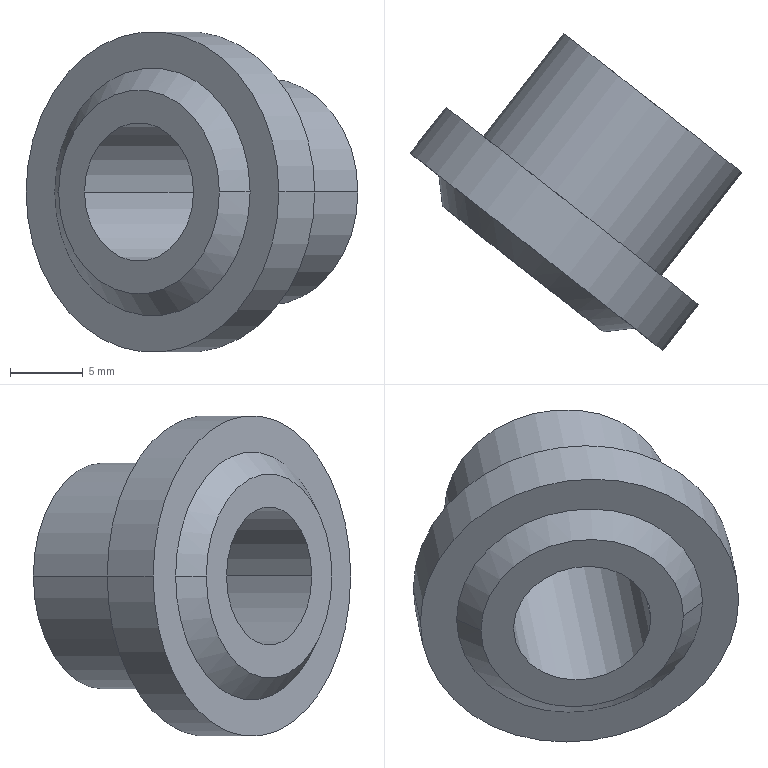Part | STEP file | VALVE_2PARTV11 | 1 solid | 12 faces | box 22.76 x 21.764 x 22 mm | volume 2471 mm3 | cylinder 6 | plane 4 | cone 2 | commonest cylinder face diameters 9.5 x2 15.5 x2 22 x2
STEP:
#1=CARTESIAN_POINT('',(0.,0.,0.));
#2=DIRECTION('',(0.,0.,1.));
#3=DIRECTION('',(1.,0.,0.));
#4=AXIS2_PLACEMENT_3D('',#1,#2,#3);
#5=CARTESIAN_POINT('',(-4.617,4.509,0.));
#6=VERTEX_POINT('',#5);
#7=CARTESIAN_POINT('',(12.719,-9.035,0.));
#8=VERTEX_POINT('',#7);
#9=CARTESIAN_POINT('',(4.051,-2.263,0.));
#10=DIRECTION('',(0.6157,0.788,0.));
#11=DIRECTION('',(-0.788,0.6157,0.));
#12=AXIS2_PLACEMENT_3D('',#9,#10,#11);
#13=CIRCLE('',#12,11.);
#14=CARTESIAN_POINT('',(2.204,-4.627,0.));
#15=DIRECTION('',(0.6157,0.788,0.));
#16=DIRECTION('',(-0.788,0.6157,0.));
#17=AXIS2_PLACEMENT_3D('',#14,#15,#16);
#18=CYLINDRICAL_SURFACE('',#17,11.);
#19=CARTESIAN_POINT('',(0.,3.));
#20=DIRECTION('',(1.,0.));
#21=VECTOR('',#20,1.);
#22=LINE('',#19,#21);
#23=(GEOMETRIC_REPRESENTATION_CONTEXT(2)PARAMETRIC_REPRESENTATION_CONTEXT()REPRESENTATION_CONTEXT('',''));
#24=DEFINITIONAL_REPRESENTATION('',(#22),#23);
#25=PCURVE('',#18,#24);
#26=CARTESIAN_POINT('',(-4.617,4.509,0.));
#27=DIRECTION('',(-0.6157,-0.788,0.));
#28=DIRECTION('',(0.788,-0.6157,0.));
#29=AXIS2_PLACEMENT_3D('',#26,#27,#28);
#30=PLANE('',#29);
#31=CARTESIAN_POINT('',(0.,0.));
#32=CARTESIAN_POINT('',(0.,19.053));
#33=CARTESIAN_POINT('',(16.5,9.526));
#34=CARTESIAN_POINT('',(33.,0.));
#35=CARTESIAN_POINT('',(16.5,-9.526));
#36=CARTESIAN_POINT('',(0.,-19.053));
#37=CARTESIAN_POINT('',(0.,0.));
#38=(BOUNDED_CURVE()B_SPLINE_CURVE(2,(#31,#32,#33,#34,#35,#36,#37),.UNSPECIFIED.,.T.,.F.)B_SPLINE_CURVE_WITH_KNOTS((1,2,2,2,2,1),(-2.094,0.,2.094,4.189,6.283,8.378),.UNSPECIFIED.)CURVE()GEOMETRIC_REPRESENTATION_ITEM()RATIONAL_B_SPLINE_CURVE((1.,0.5,1.,0.5,1.,0.5,1.))REPRESENTATION_ITEM(''));
#39=(GEOMETRIC_REPRESENTATION_CONTEXT(2)PARAMETRIC_REPRESENTATION_CONTEXT()REPRESENTATION_CONTEXT('',''));
#40=DEFINITIONAL_REPRESENTATION('',(#38),#39);
#41=PCURVE('',#30,#40);
#42=SURFACE_CURVE('',#13,(#25,#41),.PCURVE_S1.);
#43=EDGE_CURVE('',#6,#8,#42,.T.);
#44=ORIENTED_EDGE('',*,*,#43,.T.);
#45=CARTESIAN_POINT('',(15.182,-5.883,0.));
#46=VERTEX_POINT('',#45);
#47=CARTESIAN_POINT('',(10.872,-11.399,0.));
#48=DIRECTION('',(0.6157,0.788,0.));
#49=VECTOR('',#48,1.);
#50=LINE('',#47,#49);
#51=CARTESIAN_POINT('',(3.142,0.));
#52=DIRECTION('',(0.,1.));
#53=VECTOR('',#52,1.);
#54=LINE('',#51,#53);
#55=(GEOMETRIC_REPRESENTATION_CONTEXT(2)PARAMETRIC_REPRESENTATION_CONTEXT()REPRESENTATION_CONTEXT('',''));
#56=DEFINITIONAL_REPRESENTATION('',(#54),#55);
#57=PCURVE('',#18,#56);
#58=CARTESIAN_POINT('',(2.204,-4.627,0.));
#59=DIRECTION('',(0.6157,0.788,0.));
#60=DIRECTION('',(-0.788,0.6157,0.));
#61=AXIS2_PLACEMENT_3D('',#58,#59,#60);
#62=CYLINDRICAL_SURFACE('',#61,11.);
#63=CARTESIAN_POINT('',(3.142,0.));
#64=DIRECTION('',(0.,1.));
#65=VECTOR('',#64,1.);
#66=LINE('',#63,#65);
#67=(GEOMETRIC_REPRESENTATION_CONTEXT(2)PARAMETRIC_REPRESENTATION_CONTEXT()REPRESENTATION_CONTEXT('',''));
#68=DEFINITIONAL_REPRESENTATION('',(#66),#67);
#69=PCURVE('',#62,#68);
#70=SURFACE_CURVE('',#50,(#57,#69),.PCURVE_S1.);
#71=EDGE_CURVE('',#8,#46,#70,.T.);
#72=ORIENTED_EDGE('',*,*,#71,.T.);
#73=CARTESIAN_POINT('',(-2.155,7.661,0.));
#74=VERTEX_POINT('',#73);
#75=CARTESIAN_POINT('',(6.513,0.889,0.));
#76=DIRECTION('',(0.6157,0.788,0.));
#77=DIRECTION('',(-0.788,0.6157,0.));
#78=AXIS2_PLACEMENT_3D('',#75,#76,#77);
#79=CIRCLE('',#78,11.);
#80=CARTESIAN_POINT('',(0.,7.));
#81=DIRECTION('',(1.,0.));
#82=VECTOR('',#81,1.);
#83=LINE('',#80,#82);
#84=(GEOMETRIC_REPRESENTATION_CONTEXT(2)PARAMETRIC_REPRESENTATION_CONTEXT()REPRESENTATION_CONTEXT('',''));
#85=DEFINITIONAL_REPRESENTATION('',(#83),#84);
#86=PCURVE('',#18,#85);
#87=CARTESIAN_POINT('',(0.4063,5.66,0.));
#88=DIRECTION('',(0.6157,0.788,0.));
#89=DIRECTION('',(-0.788,0.6157,0.));
#90=AXIS2_PLACEMENT_3D('',#87,#88,#89);
#91=PLANE('',#90);
#92=CARTESIAN_POINT('',(-7.75,0.));
#93=DIRECTION('',(1.,0.));
#94=AXIS2_PLACEMENT_2D('',#92,#93);
#95=CIRCLE('',#94,11.);
#96=(GEOMETRIC_REPRESENTATION_CONTEXT(2)PARAMETRIC_REPRESENTATION_CONTEXT()REPRESENTATION_CONTEXT('',''));
#97=DEFINITIONAL_REPRESENTATION('',(#95),#96);
#98=PCURVE('',#91,#97);
#99=SURFACE_CURVE('',#79,(#86,#98),.PCURVE_S1.);
#100=EDGE_CURVE('',#74,#46,#99,.T.);
#101=ORIENTED_EDGE('',*,*,#100,.F.);
#102=CARTESIAN_POINT('',(-6.464,2.145,0.));
#103=DIRECTION('',(0.6157,0.788,0.));
#104=VECTOR('',#103,1.);
#105=LINE('',#102,#104);
#106=CARTESIAN_POINT('',(0.,0.));
#107=DIRECTION('',(0.,1.));
#108=VECTOR('',#107,1.);
#109=LINE('',#106,#108);
#110=(GEOMETRIC_REPRESENTATION_CONTEXT(2)PARAMETRIC_REPRESENTATION_CONTEXT()REPRESENTATION_CONTEXT('',''));
#111=DEFINITIONAL_REPRESENTATION('',(#109),#110);
#112=PCURVE('',#18,#111);
#113=CARTESIAN_POINT('',(6.283,0.));
#114=DIRECTION('',(0.,1.));
#115=VECTOR('',#114,1.);
#116=LINE('',#113,#115);
#117=(GEOMETRIC_REPRESENTATION_CONTEXT(2)PARAMETRIC_REPRESENTATION_CONTEXT()REPRESENTATION_CONTEXT('',''));
#118=DEFINITIONAL_REPRESENTATION('',(#116),#117);
#119=PCURVE('',#62,#118);
#120=SURFACE_CURVE('',#105,(#112,#119),.PCURVE_S1.);
#121=EDGE_CURVE('',#6,#74,#120,.T.);
#122=ORIENTED_EDGE('',*,*,#121,.F.);
#123=EDGE_LOOP('',(#44,#72,#101,#122));
#124=FACE_BOUND('',#123,.T.);
#125=ADVANCED_FACE('',(#124),#18,.T.);
#126=CARTESIAN_POINT('',(0.4063,5.66,0.));
#127=VERTEX_POINT('',#126);
#128=CARTESIAN_POINT('',(12.62,-3.882,0.));
#129=VERTEX_POINT('',#128);
#130=CARTESIAN_POINT('',(6.513,0.889,0.));
#131=DIRECTION('',(0.6157,0.788,0.));
#132=DIRECTION('',(-0.788,0.6157,0.));
#133=AXIS2_PLACEMENT_3D('',#130,#131,#132);
#134=CIRCLE('',#133,7.75);
#135=CARTESIAN_POINT('',(2.204,-4.627,0.));
#136=DIRECTION('',(0.6157,0.788,0.));
#137=DIRECTION('',(-0.788,0.6157,0.));
#138=AXIS2_PLACEMENT_3D('',#135,#136,#137);
#139=CYLINDRICAL_SURFACE('',#138,7.75);
#140=CARTESIAN_POINT('',(0.,7.));
#141=DIRECTION('',(1.,0.));
#142=VECTOR('',#141,1.);
#143=LINE('',#140,#142);
#144=(GEOMETRIC_REPRESENTATION_CONTEXT(2)PARAMETRIC_REPRESENTATION_CONTEXT()REPRESENTATION_CONTEXT('',''));
#145=DEFINITIONAL_REPRESENTATION('',(#143),#144);
#146=PCURVE('',#139,#145);
#147=CARTESIAN_POINT('',(-7.75,0.));
#148=DIRECTION('',(1.,0.));
#149=AXIS2_PLACEMENT_2D('',#147,#148);
#150=CIRCLE('',#149,7.75);
#151=(GEOMETRIC_REPRESENTATION_CONTEXT(2)PARAMETRIC_REPRESENTATION_CONTEXT()REPRESENTATION_CONTEXT('',''));
#152=DEFINITIONAL_REPRESENTATION('',(#150),#151);
#153=PCURVE('',#91,#152);
#154=SURFACE_CURVE('',#134,(#146,#153),.PCURVE_S1.);
#155=EDGE_CURVE('',#127,#129,#154,.T.);
#156=ORIENTED_EDGE('',*,*,#155,.T.);
#157=CARTESIAN_POINT('',(18.143,3.186,0.));
#158=VERTEX_POINT('',#157);
#159=CARTESIAN_POINT('',(8.311,-9.398,0.));
#160=DIRECTION('',(0.6157,0.788,0.));
#161=VECTOR('',#160,1.);
#162=LINE('',#159,#161);
#163=CARTESIAN_POINT('',(3.142,0.));
#164=DIRECTION('',(0.,1.));
#165=VECTOR('',#164,1.);
#166=LINE('',#163,#165);
#167=(GEOMETRIC_REPRESENTATION_CONTEXT(2)PARAMETRIC_REPRESENTATION_CONTEXT()REPRESENTATION_CONTEXT('',''));
#168=DEFINITIONAL_REPRESENTATION('',(#166),#167);
#169=PCURVE('',#139,#168);
#170=CARTESIAN_POINT('',(2.204,-4.627,0.));
#171=DIRECTION('',(0.6157,0.788,0.));
#172=DIRECTION('',(-0.788,0.6157,0.));
#173=AXIS2_PLACEMENT_3D('',#170,#171,#172);
#174=CYLINDRICAL_SURFACE('',#173,7.75);
#175=CARTESIAN_POINT('',(3.142,0.));
#176=DIRECTION('',(0.,1.));
#177=VECTOR('',#176,1.);
#178=LINE('',#175,#177);
#179=(GEOMETRIC_REPRESENTATION_CONTEXT(2)PARAMETRIC_REPRESENTATION_CONTEXT()REPRESENTATION_CONTEXT('',''));
#180=DEFINITIONAL_REPRESENTATION('',(#178),#179);
#181=PCURVE('',#174,#180);
#182=SURFACE_CURVE('',#162,(#169,#181),.PCURVE_S1.);
#183=EDGE_CURVE('',#129,#158,#182,.T.);
#184=ORIENTED_EDGE('',*,*,#183,.T.);
#185=CARTESIAN_POINT('',(5.929,12.728,0.));
#186=VERTEX_POINT('',#185);
#187=CARTESIAN_POINT('',(12.036,7.957,0.));
#188=DIRECTION('',(0.6157,0.788,0.));
#189=DIRECTION('',(-0.788,0.6157,0.));
#190=AXIS2_PLACEMENT_3D('',#187,#188,#189);
#191=CIRCLE('',#190,7.75);
#192=CARTESIAN_POINT('',(0.,15.97));
#193=DIRECTION('',(1.,0.));
#194=VECTOR('',#193,1.);
#195=LINE('',#192,#194);
#196=(GEOMETRIC_REPRESENTATION_CONTEXT(2)PARAMETRIC_REPRESENTATION_CONTEXT()REPRESENTATION_CONTEXT('',''));
#197=DEFINITIONAL_REPRESENTATION('',(#195),#196);
#198=PCURVE('',#139,#197);
#199=CARTESIAN_POINT('',(8.293,10.882,0.));
#200=DIRECTION('',(0.6157,0.788,0.));
#201=DIRECTION('',(-0.788,0.6157,0.));
#202=AXIS2_PLACEMENT_3D('',#199,#200,#201);
#203=PLANE('',#202);
#204=CARTESIAN_POINT('',(-4.75,0.));
#205=DIRECTION('',(1.,0.));
#206=AXIS2_PLACEMENT_2D('',#204,#205);
#207=CIRCLE('',#206,7.75);
#208=(GEOMETRIC_REPRESENTATION_CONTEXT(2)PARAMETRIC_REPRESENTATION_CONTEXT()REPRESENTATION_CONTEXT('',''));
#209=DEFINITIONAL_REPRESENTATION('',(#207),#208);
#210=PCURVE('',#203,#209);
#211=SURFACE_CURVE('',#191,(#198,#210),.PCURVE_S1.);
#212=EDGE_CURVE('',#186,#158,#211,.T.);
#213=ORIENTED_EDGE('',*,*,#212,.F.);
#214=CARTESIAN_POINT('',(-3.903,0.1443,0.));
#215=DIRECTION('',(0.6157,0.788,0.));
#216=VECTOR('',#215,1.);
#217=LINE('',#214,#216);
#218=CARTESIAN_POINT('',(0.,0.));
#219=DIRECTION('',(0.,1.));
#220=VECTOR('',#219,1.);
#221=LINE('',#218,#220);
#222=(GEOMETRIC_REPRESENTATION_CONTEXT(2)PARAMETRIC_REPRESENTATION_CONTEXT()REPRESENTATION_CONTEXT('',''));
#223=DEFINITIONAL_REPRESENTATION('',(#221),#222);
#224=PCURVE('',#139,#223);
#225=CARTESIAN_POINT('',(6.283,0.));
#226=DIRECTION('',(0.,1.));
#227=VECTOR('',#226,1.);
#228=LINE('',#225,#227);
#229=(GEOMETRIC_REPRESENTATION_CONTEXT(2)PARAMETRIC_REPRESENTATION_CONTEXT()REPRESENTATION_CONTEXT('',''));
#230=DEFINITIONAL_REPRESENTATION('',(#228),#229);
#231=PCURVE('',#174,#230);
#232=SURFACE_CURVE('',#217,(#224,#231),.PCURVE_S1.);
#233=EDGE_CURVE('',#127,#186,#232,.T.);
#234=ORIENTED_EDGE('',*,*,#233,.F.);
#235=EDGE_LOOP('',(#156,#184,#213,#234));
#236=FACE_BOUND('',#235,.T.);
#237=ADVANCED_FACE('',(#236),#139,.T.);
#238=CARTESIAN_POINT('',(-0.6158,-0.5207,0.));
#239=VERTEX_POINT('',#238);
#240=CARTESIAN_POINT('',(8.293,10.882,0.));
#241=VERTEX_POINT('',#240);
#242=CARTESIAN_POINT('',(-1.539,-1.703,0.));
#243=DIRECTION('',(0.6157,0.788,0.));
#244=VECTOR('',#243,1.);
#245=LINE('',#242,#244);
#246=CARTESIAN_POINT('',(2.204,-4.627,0.));
#247=DIRECTION('',(0.6157,0.788,0.));
#248=DIRECTION('',(-0.788,0.6157,0.));
#249=AXIS2_PLACEMENT_3D('',#246,#247,#248);
#250=CYLINDRICAL_SURFACE('',#249,4.75);
#251=CARTESIAN_POINT('',(6.283,0.));
#252=DIRECTION('',(0.,1.));
#253=VECTOR('',#252,1.);
#254=LINE('',#251,#253);
#255=(GEOMETRIC_REPRESENTATION_CONTEXT(2)PARAMETRIC_REPRESENTATION_CONTEXT()REPRESENTATION_CONTEXT('',''));
#256=DEFINITIONAL_REPRESENTATION('',(#254),#255);
#257=PCURVE('',#250,#256);
#258=CARTESIAN_POINT('',(2.204,-4.627,0.));
#259=DIRECTION('',(0.6157,0.788,0.));
#260=DIRECTION('',(-0.788,0.6157,0.));
#261=AXIS2_PLACEMENT_3D('',#258,#259,#260);
#262=CYLINDRICAL_SURFACE('',#261,4.75);
#263=CARTESIAN_POINT('',(0.,0.));
#264=DIRECTION('',(0.,1.));
#265=VECTOR('',#264,1.);
#266=LINE('',#263,#265);
#267=(GEOMETRIC_REPRESENTATION_CONTEXT(2)PARAMETRIC_REPRESENTATION_CONTEXT()REPRESENTATION_CONTEXT('',''));
#268=DEFINITIONAL_REPRESENTATION('',(#266),#267);
#269=PCURVE('',#262,#268);
#270=SURFACE_CURVE('',#245,(#257,#269),.PCURVE_S1.);
#271=EDGE_CURVE('',#239,#241,#270,.T.);
#272=ORIENTED_EDGE('',*,*,#271,.T.);
#273=CARTESIAN_POINT('',(15.779,5.033,0.));
#274=VERTEX_POINT('',#273);
#275=CARTESIAN_POINT('',(12.036,7.957,0.));
#276=DIRECTION('',(0.6157,0.788,0.));
#277=DIRECTION('',(-0.788,0.6157,0.));
#278=AXIS2_PLACEMENT_3D('',#275,#276,#277);
#279=CIRCLE('',#278,4.75);
#280=CARTESIAN_POINT('',(0.,15.97));
#281=DIRECTION('',(1.,0.));
#282=VECTOR('',#281,1.);
#283=LINE('',#280,#282);
#284=(GEOMETRIC_REPRESENTATION_CONTEXT(2)PARAMETRIC_REPRESENTATION_CONTEXT()REPRESENTATION_CONTEXT('',''));
#285=DEFINITIONAL_REPRESENTATION('',(#283),#284);
#286=PCURVE('',#250,#285);
#287=CARTESIAN_POINT('',(-4.75,0.));
#288=DIRECTION('',(1.,0.));
#289=AXIS2_PLACEMENT_2D('',#287,#288);
#290=CIRCLE('',#289,4.75);
#291=(GEOMETRIC_REPRESENTATION_CONTEXT(2)PARAMETRIC_REPRESENTATION_CONTEXT()REPRESENTATION_CONTEXT('',''));
#292=DEFINITIONAL_REPRESENTATION('',(#290),#291);
#293=PCURVE('',#203,#292);
#294=SURFACE_CURVE('',#279,(#286,#293),.PCURVE_S1.);
#295=EDGE_CURVE('',#274,#241,#294,.T.);
#296=ORIENTED_EDGE('',*,*,#295,.F.);
#297=CARTESIAN_POINT('',(6.87,-6.369,0.));
#298=VERTEX_POINT('',#297);
#299=CARTESIAN_POINT('',(5.947,-7.551,0.));
#300=DIRECTION('',(0.6157,0.788,0.));
#301=VECTOR('',#300,1.);
#302=LINE('',#299,#301);
#303=CARTESIAN_POINT('',(3.142,0.));
#304=DIRECTION('',(0.,1.));
#305=VECTOR('',#304,1.);
#306=LINE('',#303,#305);
#307=(GEOMETRIC_REPRESENTATION_CONTEXT(2)PARAMETRIC_REPRESENTATION_CONTEXT()REPRESENTATION_CONTEXT('',''));
#308=DEFINITIONAL_REPRESENTATION('',(#306),#307);
#309=PCURVE('',#250,#308);
#310=CARTESIAN_POINT('',(3.142,0.));
#311=DIRECTION('',(0.,1.));
#312=VECTOR('',#311,1.);
#313=LINE('',#310,#312);
#314=(GEOMETRIC_REPRESENTATION_CONTEXT(2)PARAMETRIC_REPRESENTATION_CONTEXT()REPRESENTATION_CONTEXT('',''));
#315=DEFINITIONAL_REPRESENTATION('',(#313),#314);
#316=PCURVE('',#262,#315);
#317=SURFACE_CURVE('',#302,(#309,#316),.PCURVE_S1.);
#318=EDGE_CURVE('',#298,#274,#317,.T.);
#319=ORIENTED_EDGE('',*,*,#318,.F.);
#320=CARTESIAN_POINT('',(3.127,-3.445,0.));
#321=DIRECTION('',(0.6157,0.788,0.));
#322=DIRECTION('',(-0.788,0.6157,0.));
#323=AXIS2_PLACEMENT_3D('',#320,#321,#322);
#324=CIRCLE('',#323,4.75);
#325=CARTESIAN_POINT('',(0.,1.5));
#326=DIRECTION('',(1.,0.));
#327=VECTOR('',#326,1.);
#328=LINE('',#325,#327);
#329=(GEOMETRIC_REPRESENTATION_CONTEXT(2)PARAMETRIC_REPRESENTATION_CONTEXT()REPRESENTATION_CONTEXT('',''));
#330=DEFINITIONAL_REPRESENTATION('',(#328),#329);
#331=PCURVE('',#250,#330);
#332=CARTESIAN_POINT('',(-2.389,0.8645,0.));
#333=DIRECTION('',(-0.6157,-0.788,0.));
#334=DIRECTION('',(0.788,-0.6157,0.));
#335=AXIS2_PLACEMENT_3D('',#332,#333,#334);
#336=PLANE('',#335);
#337=CARTESIAN_POINT('',(2.25,0.));
#338=CARTESIAN_POINT('',(2.25,8.227));
#339=CARTESIAN_POINT('',(9.375,4.114));
#340=CARTESIAN_POINT('',(16.5,0.));
#341=CARTESIAN_POINT('',(9.375,-4.114));
#342=CARTESIAN_POINT('',(2.25,-8.227));
#343=CARTESIAN_POINT('',(2.25,0.));
#344=(BOUNDED_CURVE()B_SPLINE_CURVE(2,(#337,#338,#339,#340,#341,#342,#343),.UNSPECIFIED.,.T.,.F.)B_SPLINE_CURVE_WITH_KNOTS((1,2,2,2,2,1),(-2.094,0.,2.094,4.189,6.283,8.378),.UNSPECIFIED.)CURVE()GEOMETRIC_REPRESENTATION_ITEM()RATIONAL_B_SPLINE_CURVE((1.,0.5,1.,0.5,1.,0.5,1.))REPRESENTATION_ITEM(''));
#345=(GEOMETRIC_REPRESENTATION_CONTEXT(2)PARAMETRIC_REPRESENTATION_CONTEXT()REPRESENTATION_CONTEXT('',''));
#346=DEFINITIONAL_REPRESENTATION('',(#344),#345);
#347=PCURVE('',#336,#346);
#348=SURFACE_CURVE('',#324,(#331,#347),.PCURVE_S1.);
#349=EDGE_CURVE('',#298,#239,#348,.T.);
#350=ORIENTED_EDGE('',*,*,#349,.T.);
#351=EDGE_LOOP('',(#272,#296,#319,#350));
#352=FACE_BOUND('',#351,.F.);
#353=ADVANCED_FACE('',(#352),#250,.F.);
#354=CARTESIAN_POINT('',(-2.389,0.8645,0.));
#355=VERTEX_POINT('',#354);
#356=CARTESIAN_POINT('',(8.643,-7.755,0.));
#357=VERTEX_POINT('',#356);
#358=CARTESIAN_POINT('',(3.127,-3.445,0.));
#359=DIRECTION('',(0.6157,0.788,0.));
#360=DIRECTION('',(-0.788,0.6157,0.));
#361=AXIS2_PLACEMENT_3D('',#358,#359,#360);
#362=CIRCLE('',#361,7.);
#363=CARTESIAN_POINT('',(4.051,-2.263,0.));
#364=DIRECTION('',(0.6157,0.788,0.));
#365=DIRECTION('',(-0.788,0.6157,0.));
#366=AXIS2_PLACEMENT_3D('',#363,#364,#365);
#367=CONICAL_SURFACE('',#366,8.5,0.7854);
#368=CARTESIAN_POINT('',(0.,-1.5));
#369=DIRECTION('',(1.,0.));
#370=VECTOR('',#369,1.);
#371=LINE('',#368,#370);
#372=(GEOMETRIC_REPRESENTATION_CONTEXT(2)PARAMETRIC_REPRESENTATION_CONTEXT()REPRESENTATION_CONTEXT('',''));
#373=DEFINITIONAL_REPRESENTATION('',(#371),#372);
#374=PCURVE('',#367,#373);
#375=CARTESIAN_POINT('',(0.,0.));
#376=CARTESIAN_POINT('',(0.,12.124));
#377=CARTESIAN_POINT('',(10.5,6.062));
#378=CARTESIAN_POINT('',(21.,0.));
#379=CARTESIAN_POINT('',(10.5,-6.062));
#380=CARTESIAN_POINT('',(0.,-12.124));
#381=CARTESIAN_POINT('',(0.,0.));
#382=(BOUNDED_CURVE()B_SPLINE_CURVE(2,(#375,#376,#377,#378,#379,#380,#381),.UNSPECIFIED.,.T.,.F.)B_SPLINE_CURVE_WITH_KNOTS((1,2,2,2,2,1),(-2.094,0.,2.094,4.189,6.283,8.378),.UNSPECIFIED.)CURVE()GEOMETRIC_REPRESENTATION_ITEM()RATIONAL_B_SPLINE_CURVE((1.,0.5,1.,0.5,1.,0.5,1.))REPRESENTATION_ITEM(''));
#383=(GEOMETRIC_REPRESENTATION_CONTEXT(2)PARAMETRIC_REPRESENTATION_CONTEXT()REPRESENTATION_CONTEXT('',''));
#384=DEFINITIONAL_REPRESENTATION('',(#382),#383);
#385=PCURVE('',#336,#384);
#386=SURFACE_CURVE('',#362,(#374,#385),.PCURVE_S1.);
#387=EDGE_CURVE('',#355,#357,#386,.T.);
#388=ORIENTED_EDGE('',*,*,#387,.T.);
#389=CARTESIAN_POINT('',(10.749,-7.496,0.));
#390=VERTEX_POINT('',#389);
#391=CARTESIAN_POINT('',(10.749,-7.496,0.));
#392=DIRECTION('',(0.9925,0.1219,0.));
#393=VECTOR('',#392,1.);
#394=LINE('',#391,#393);
#395=CARTESIAN_POINT('',(3.142,0.));
#396=DIRECTION('',(0.,1.));
#397=VECTOR('',#396,1.);
#398=LINE('',#395,#397);
#399=(GEOMETRIC_REPRESENTATION_CONTEXT(2)PARAMETRIC_REPRESENTATION_CONTEXT()REPRESENTATION_CONTEXT('',''));
#400=DEFINITIONAL_REPRESENTATION('',(#398),#399);
#401=PCURVE('',#367,#400);
#402=CARTESIAN_POINT('',(4.051,-2.263,0.));
#403=DIRECTION('',(0.6157,0.788,0.));
#404=DIRECTION('',(-0.788,0.6157,0.));
#405=AXIS2_PLACEMENT_3D('',#402,#403,#404);
#406=CONICAL_SURFACE('',#405,8.5,0.7854);
#407=CARTESIAN_POINT('',(3.142,0.));
#408=DIRECTION('',(0.,1.));
#409=VECTOR('',#408,1.);
#410=LINE('',#407,#409);
#411=(GEOMETRIC_REPRESENTATION_CONTEXT(2)PARAMETRIC_REPRESENTATION_CONTEXT()REPRESENTATION_CONTEXT('',''));
#412=DEFINITIONAL_REPRESENTATION('',(#410),#411);
#413=PCURVE('',#406,#412);
#414=SURFACE_CURVE('',#394,(#401,#413),.PCURVE_S1.);
#415=EDGE_CURVE('',#357,#390,#414,.T.);
#416=ORIENTED_EDGE('',*,*,#415,.T.);
#417=CARTESIAN_POINT('',(-2.647,2.97,0.));
#418=VERTEX_POINT('',#417);
#419=CARTESIAN_POINT('',(4.051,-2.263,0.));
#420=DIRECTION('',(0.6157,0.788,0.));
#421=DIRECTION('',(-0.788,0.6157,0.));
#422=AXIS2_PLACEMENT_3D('',#419,#420,#421);
#423=CIRCLE('',#422,8.5);
#424=CARTESIAN_POINT('',(0.,0.));
#425=DIRECTION('',(1.,0.));
#426=VECTOR('',#425,1.);
#427=LINE('',#424,#426);
#428=(GEOMETRIC_REPRESENTATION_CONTEXT(2)PARAMETRIC_REPRESENTATION_CONTEXT()REPRESENTATION_CONTEXT('',''));
#429=DEFINITIONAL_REPRESENTATION('',(#427),#428);
#430=PCURVE('',#367,#429);
#431=CARTESIAN_POINT('',(2.5,0.));
#432=CARTESIAN_POINT('',(2.5,14.722));
#433=CARTESIAN_POINT('',(15.25,7.361));
#434=CARTESIAN_POINT('',(28.,0.));
#435=CARTESIAN_POINT('',(15.25,-7.361));
#436=CARTESIAN_POINT('',(2.5,-14.722));
#437=CARTESIAN_POINT('',(2.5,0.));
#438=(BOUNDED_CURVE()B_SPLINE_CURVE(2,(#431,#432,#433,#434,#435,#436,#437),.UNSPECIFIED.,.T.,.F.)B_SPLINE_CURVE_WITH_KNOTS((1,2,2,2,2,1),(-2.094,0.,2.094,4.189,6.283,8.378),.UNSPECIFIED.)CURVE()GEOMETRIC_REPRESENTATION_ITEM()RATIONAL_B_SPLINE_CURVE((1.,0.5,1.,0.5,1.,0.5,1.))REPRESENTATION_ITEM(''));
#439=(GEOMETRIC_REPRESENTATION_CONTEXT(2)PARAMETRIC_REPRESENTATION_CONTEXT()REPRESENTATION_CONTEXT('',''));
#440=DEFINITIONAL_REPRESENTATION('',(#438),#439);
#441=PCURVE('',#30,#440);
#442=SURFACE_CURVE('',#423,(#430,#441),.PCURVE_S1.);
#443=EDGE_CURVE('',#418,#390,#442,.T.);
#444=ORIENTED_EDGE('',*,*,#443,.F.);
#445=CARTESIAN_POINT('',(-2.647,2.97,0.));
#446=DIRECTION('',(-0.1219,0.9925,0.));
#447=VECTOR('',#446,1.);
#448=LINE('',#445,#447);
#449=CARTESIAN_POINT('',(0.,0.));
#450=DIRECTION('',(0.,1.));
#451=VECTOR('',#450,1.);
#452=LINE('',#449,#451);
#453=(GEOMETRIC_REPRESENTATION_CONTEXT(2)PARAMETRIC_REPRESENTATION_CONTEXT()REPRESENTATION_CONTEXT('',''));
#454=DEFINITIONAL_REPRESENTATION('',(#452),#453);
#455=PCURVE('',#367,#454);
#456=CARTESIAN_POINT('',(6.283,0.));
#457=DIRECTION('',(0.,1.));
#458=VECTOR('',#457,1.);
#459=LINE('',#456,#458);
#460=(GEOMETRIC_REPRESENTATION_CONTEXT(2)PARAMETRIC_REPRESENTATION_CONTEXT()REPRESENTATION_CONTEXT('',''));
#461=DEFINITIONAL_REPRESENTATION('',(#459),#460);
#462=PCURVE('',#406,#461);
#463=SURFACE_CURVE('',#448,(#455,#462),.PCURVE_S1.);
#464=EDGE_CURVE('',#355,#418,#463,.T.);
#465=ORIENTED_EDGE('',*,*,#464,.F.);
#466=EDGE_LOOP('',(#388,#416,#444,#465));
#467=FACE_BOUND('',#466,.T.);
#468=ADVANCED_FACE('',(#467),#367,.T.);
#469=ORIENTED_EDGE('',*,*,#415,.F.);
#470=CARTESIAN_POINT('',(3.127,-3.445,0.));
#471=DIRECTION('',(0.6157,0.788,0.));
#472=DIRECTION('',(-0.788,0.6157,0.));
#473=AXIS2_PLACEMENT_3D('',#470,#471,#472);
#474=CIRCLE('',#473,7.);
#475=CARTESIAN_POINT('',(0.,-1.5));
#476=DIRECTION('',(1.,0.));
#477=VECTOR('',#476,1.);
#478=LINE('',#475,#477);
#479=(GEOMETRIC_REPRESENTATION_CONTEXT(2)PARAMETRIC_REPRESENTATION_CONTEXT()REPRESENTATION_CONTEXT('',''));
#480=DEFINITIONAL_REPRESENTATION('',(#478),#479);
#481=PCURVE('',#406,#480);
#482=CARTESIAN_POINT('',(0.,0.));
#483=CARTESIAN_POINT('',(0.,12.124));
#484=CARTESIAN_POINT('',(10.5,6.062));
#485=CARTESIAN_POINT('',(21.,0.));
#486=CARTESIAN_POINT('',(10.5,-6.062));
#487=CARTESIAN_POINT('',(0.,-12.124));
#488=CARTESIAN_POINT('',(0.,0.));
#489=(BOUNDED_CURVE()B_SPLINE_CURVE(2,(#482,#483,#484,#485,#486,#487,#488),.UNSPECIFIED.,.T.,.F.)B_SPLINE_CURVE_WITH_KNOTS((1,2,2,2,2,1),(-2.094,0.,2.094,4.189,6.283,8.378),.UNSPECIFIED.)CURVE()GEOMETRIC_REPRESENTATION_ITEM()RATIONAL_B_SPLINE_CURVE((1.,0.5,1.,0.5,1.,0.5,1.))REPRESENTATION_ITEM(''));
#490=(GEOMETRIC_REPRESENTATION_CONTEXT(2)PARAMETRIC_REPRESENTATION_CONTEXT()REPRESENTATION_CONTEXT('',''));
#491=DEFINITIONAL_REPRESENTATION('',(#489),#490);
#492=PCURVE('',#336,#491);
#493=SURFACE_CURVE('',#474,(#481,#492),.PCURVE_S1.);
#494=EDGE_CURVE('',#357,#355,#493,.T.);
#495=ORIENTED_EDGE('',*,*,#494,.T.);
#496=ORIENTED_EDGE('',*,*,#464,.T.);
#497=CARTESIAN_POINT('',(4.051,-2.263,0.));
#498=DIRECTION('',(0.6157,0.788,0.));
#499=DIRECTION('',(-0.788,0.6157,0.));
#500=AXIS2_PLACEMENT_3D('',#497,#498,#499);
#501=CIRCLE('',#500,8.5);
#502=CARTESIAN_POINT('',(0.,0.));
#503=DIRECTION('',(1.,0.));
#504=VECTOR('',#503,1.);
#505=LINE('',#502,#504);
#506=(GEOMETRIC_REPRESENTATION_CONTEXT(2)PARAMETRIC_REPRESENTATION_CONTEXT()REPRESENTATION_CONTEXT('',''));
#507=DEFINITIONAL_REPRESENTATION('',(#505),#506);
#508=PCURVE('',#406,#507);
#509=CARTESIAN_POINT('',(2.5,0.));
#510=CARTESIAN_POINT('',(2.5,14.722));
#511=CARTESIAN_POINT('',(15.25,7.361));
#512=CARTESIAN_POINT('',(28.,0.));
#513=CARTESIAN_POINT('',(15.25,-7.361));
#514=CARTESIAN_POINT('',(2.5,-14.722));
#515=CARTESIAN_POINT('',(2.5,0.));
#516=(BOUNDED_CURVE()B_SPLINE_CURVE(2,(#509,#510,#511,#512,#513,#514,#515),.UNSPECIFIED.,.T.,.F.)B_SPLINE_CURVE_WITH_KNOTS((1,2,2,2,2,1),(-2.094,0.,2.094,4.189,6.283,8.378),.UNSPECIFIED.)CURVE()GEOMETRIC_REPRESENTATION_ITEM()RATIONAL_B_SPLINE_CURVE((1.,0.5,1.,0.5,1.,0.5,1.))REPRESENTATION_ITEM(''));
#517=(GEOMETRIC_REPRESENTATION_CONTEXT(2)PARAMETRIC_REPRESENTATION_CONTEXT()REPRESENTATION_CONTEXT('',''));
#518=DEFINITIONAL_REPRESENTATION('',(#516),#517);
#519=PCURVE('',#30,#518);
#520=SURFACE_CURVE('',#501,(#508,#519),.PCURVE_S1.);
#521=EDGE_CURVE('',#390,#418,#520,.T.);
#522=ORIENTED_EDGE('',*,*,#521,.F.);
#523=EDGE_LOOP('',(#469,#495,#496,#522));
#524=FACE_BOUND('',#523,.T.);
#525=ADVANCED_FACE('',(#524),#406,.T.);
#526=CARTESIAN_POINT('',(3.127,-3.445,0.));
#527=DIRECTION('',(0.6157,0.788,0.));
#528=DIRECTION('',(-0.788,0.6157,0.));
#529=AXIS2_PLACEMENT_3D('',#526,#527,#528);
#530=CIRCLE('',#529,4.75);
#531=CARTESIAN_POINT('',(2.25,0.));
#532=CARTESIAN_POINT('',(2.25,8.227));
#533=CARTESIAN_POINT('',(9.375,4.114));
#534=CARTESIAN_POINT('',(16.5,0.));
#535=CARTESIAN_POINT('',(9.375,-4.114));
#536=CARTESIAN_POINT('',(2.25,-8.227));
#537=CARTESIAN_POINT('',(2.25,0.));
#538=(BOUNDED_CURVE()B_SPLINE_CURVE(2,(#531,#532,#533,#534,#535,#536,#537),.UNSPECIFIED.,.T.,.F.)B_SPLINE_CURVE_WITH_KNOTS((1,2,2,2,2,1),(-2.094,0.,2.094,4.189,6.283,8.378),.UNSPECIFIED.)CURVE()GEOMETRIC_REPRESENTATION_ITEM()RATIONAL_B_SPLINE_CURVE((1.,0.5,1.,0.5,1.,0.5,1.))REPRESENTATION_ITEM(''));
#539=(GEOMETRIC_REPRESENTATION_CONTEXT(2)PARAMETRIC_REPRESENTATION_CONTEXT()REPRESENTATION_CONTEXT('',''));
#540=DEFINITIONAL_REPRESENTATION('',(#538),#539);
#541=PCURVE('',#336,#540);
#542=CARTESIAN_POINT('',(0.,1.5));
#543=DIRECTION('',(1.,0.));
#544=VECTOR('',#543,1.);
#545=LINE('',#542,#544);
#546=(GEOMETRIC_REPRESENTATION_CONTEXT(2)PARAMETRIC_REPRESENTATION_CONTEXT()REPRESENTATION_CONTEXT('',''));
#547=DEFINITIONAL_REPRESENTATION('',(#545),#546);
#548=PCURVE('',#262,#547);
#549=SURFACE_CURVE('',#530,(#541,#548),.PCURVE_S1.);
#550=EDGE_CURVE('',#239,#298,#549,.T.);
#551=ORIENTED_EDGE('',*,*,#550,.T.);
#552=ORIENTED_EDGE('',*,*,#349,.T.);
#553=EDGE_LOOP('',(#551,#552));
#554=FACE_BOUND('',#553,.T.);
#555=ORIENTED_EDGE('',*,*,#387,.F.);
#556=ORIENTED_EDGE('',*,*,#494,.F.);
#557=EDGE_LOOP('',(#555,#556));
#558=FACE_BOUND('',#557,.T.);
#559=ADVANCED_FACE('',(#554,#558),#336,.T.);
#560=CARTESIAN_POINT('',(12.036,7.957,0.));
#561=DIRECTION('',(0.6157,0.788,0.));
#562=DIRECTION('',(-0.788,0.6157,0.));
#563=AXIS2_PLACEMENT_3D('',#560,#561,#562);
#564=CIRCLE('',#563,4.75);
#565=CARTESIAN_POINT('',(0.,15.97));
#566=DIRECTION('',(1.,0.));
#567=VECTOR('',#566,1.);
#568=LINE('',#565,#567);
#569=(GEOMETRIC_REPRESENTATION_CONTEXT(2)PARAMETRIC_REPRESENTATION_CONTEXT()REPRESENTATION_CONTEXT('',''));
#570=DEFINITIONAL_REPRESENTATION('',(#568),#569);
#571=PCURVE('',#262,#570);
#572=CARTESIAN_POINT('',(-4.75,0.));
#573=DIRECTION('',(1.,0.));
#574=AXIS2_PLACEMENT_2D('',#572,#573);
#575=CIRCLE('',#574,4.75);
#576=(GEOMETRIC_REPRESENTATION_CONTEXT(2)PARAMETRIC_REPRESENTATION_CONTEXT()REPRESENTATION_CONTEXT('',''));
#577=DEFINITIONAL_REPRESENTATION('',(#575),#576);
#578=PCURVE('',#203,#577);
#579=SURFACE_CURVE('',#564,(#571,#578),.PCURVE_S1.);
#580=EDGE_CURVE('',#241,#274,#579,.T.);
#581=ORIENTED_EDGE('',*,*,#580,.F.);
#582=ORIENTED_EDGE('',*,*,#271,.F.);
#583=ORIENTED_EDGE('',*,*,#550,.T.);
#584=ORIENTED_EDGE('',*,*,#318,.T.);
#585=EDGE_LOOP('',(#581,#582,#583,#584));
#586=FACE_BOUND('',#585,.F.);
#587=ADVANCED_FACE('',(#586),#262,.F.);
#588=ORIENTED_EDGE('',*,*,#212,.T.);
#589=CARTESIAN_POINT('',(12.036,7.957,0.));
#590=DIRECTION('',(0.6157,0.788,0.));
#591=DIRECTION('',(-0.788,0.6157,0.));
#592=AXIS2_PLACEMENT_3D('',#589,#590,#591);
#593=CIRCLE('',#592,7.75);
#594=CARTESIAN_POINT('',(-4.75,0.));
#595=DIRECTION('',(1.,0.));
#596=AXIS2_PLACEMENT_2D('',#594,#595);
#597=CIRCLE('',#596,7.75);
#598=(GEOMETRIC_REPRESENTATION_CONTEXT(2)PARAMETRIC_REPRESENTATION_CONTEXT()REPRESENTATION_CONTEXT('',''));
#599=DEFINITIONAL_REPRESENTATION('',(#597),#598);
#600=PCURVE('',#203,#599);
#601=CARTESIAN_POINT('',(0.,15.97));
#602=DIRECTION('',(1.,0.));
#603=VECTOR('',#602,1.);
#604=LINE('',#601,#603);
#605=(GEOMETRIC_REPRESENTATION_CONTEXT(2)PARAMETRIC_REPRESENTATION_CONTEXT()REPRESENTATION_CONTEXT('',''));
#606=DEFINITIONAL_REPRESENTATION('',(#604),#605);
#607=PCURVE('',#174,#606);
#608=SURFACE_CURVE('',#593,(#600,#607),.PCURVE_S1.);
#609=EDGE_CURVE('',#158,#186,#608,.T.);
#610=ORIENTED_EDGE('',*,*,#609,.T.);
#611=EDGE_LOOP('',(#588,#610));
#612=FACE_BOUND('',#611,.T.);
#613=ORIENTED_EDGE('',*,*,#580,.F.);
#614=ORIENTED_EDGE('',*,*,#295,.F.);
#615=EDGE_LOOP('',(#613,#614));
#616=FACE_BOUND('',#615,.T.);
#617=ADVANCED_FACE('',(#612,#616),#203,.T.);
#618=ORIENTED_EDGE('',*,*,#183,.F.);
#619=CARTESIAN_POINT('',(6.513,0.889,0.));
#620=DIRECTION('',(0.6157,0.788,0.));
#621=DIRECTION('',(-0.788,0.6157,0.));
#622=AXIS2_PLACEMENT_3D('',#619,#620,#621);
#623=CIRCLE('',#622,7.75);
#624=CARTESIAN_POINT('',(0.,7.));
#625=DIRECTION('',(1.,0.));
#626=VECTOR('',#625,1.);
#627=LINE('',#624,#626);
#628=(GEOMETRIC_REPRESENTATION_CONTEXT(2)PARAMETRIC_REPRESENTATION_CONTEXT()REPRESENTATION_CONTEXT('',''));
#629=DEFINITIONAL_REPRESENTATION('',(#627),#628);
#630=PCURVE('',#174,#629);
#631=CARTESIAN_POINT('',(-7.75,0.));
#632=DIRECTION('',(1.,0.));
#633=AXIS2_PLACEMENT_2D('',#631,#632);
#634=CIRCLE('',#633,7.75);
#635=(GEOMETRIC_REPRESENTATION_CONTEXT(2)PARAMETRIC_REPRESENTATION_CONTEXT()REPRESENTATION_CONTEXT('',''));
#636=DEFINITIONAL_REPRESENTATION('',(#634),#635);
#637=PCURVE('',#91,#636);
#638=SURFACE_CURVE('',#623,(#630,#637),.PCURVE_S1.);
#639=EDGE_CURVE('',#129,#127,#638,.T.);
#640=ORIENTED_EDGE('',*,*,#639,.T.);
#641=ORIENTED_EDGE('',*,*,#233,.T.);
#642=ORIENTED_EDGE('',*,*,#609,.F.);
#643=EDGE_LOOP('',(#618,#640,#641,#642));
#644=FACE_BOUND('',#643,.T.);
#645=ADVANCED_FACE('',(#644),#174,.T.);
#646=ORIENTED_EDGE('',*,*,#100,.T.);
#647=CARTESIAN_POINT('',(6.513,0.889,0.));
#648=DIRECTION('',(0.6157,0.788,0.));
#649=DIRECTION('',(-0.788,0.6157,0.));
#650=AXIS2_PLACEMENT_3D('',#647,#648,#649);
#651=CIRCLE('',#650,11.);
#652=CARTESIAN_POINT('',(-7.75,0.));
#653=DIRECTION('',(1.,0.));
#654=AXIS2_PLACEMENT_2D('',#652,#653);
#655=CIRCLE('',#654,11.);
#656=(GEOMETRIC_REPRESENTATION_CONTEXT(2)PARAMETRIC_REPRESENTATION_CONTEXT()REPRESENTATION_CONTEXT('',''));
#657=DEFINITIONAL_REPRESENTATION('',(#655),#656);
#658=PCURVE('',#91,#657);
#659=CARTESIAN_POINT('',(0.,7.));
#660=DIRECTION('',(1.,0.));
#661=VECTOR('',#660,1.);
#662=LINE('',#659,#661);
#663=(GEOMETRIC_REPRESENTATION_CONTEXT(2)PARAMETRIC_REPRESENTATION_CONTEXT()REPRESENTATION_CONTEXT('',''));
#664=DEFINITIONAL_REPRESENTATION('',(#662),#663);
#665=PCURVE('',#62,#664);
#666=SURFACE_CURVE('',#651,(#658,#665),.PCURVE_S1.);
#667=EDGE_CURVE('',#46,#74,#666,.T.);
#668=ORIENTED_EDGE('',*,*,#667,.T.);
#669=EDGE_LOOP('',(#646,#668));
#670=FACE_BOUND('',#669,.T.);
#671=ORIENTED_EDGE('',*,*,#155,.F.);
#672=ORIENTED_EDGE('',*,*,#639,.F.);
#673=EDGE_LOOP('',(#671,#672));
#674=FACE_BOUND('',#673,.T.);
#675=ADVANCED_FACE('',(#670,#674),#91,.T.);
#676=ORIENTED_EDGE('',*,*,#71,.F.);
#677=CARTESIAN_POINT('',(4.051,-2.263,0.));
#678=DIRECTION('',(0.6157,0.788,0.));
#679=DIRECTION('',(-0.788,0.6157,0.));
#680=AXIS2_PLACEMENT_3D('',#677,#678,#679);
#681=CIRCLE('',#680,11.);
#682=CARTESIAN_POINT('',(0.,3.));
#683=DIRECTION('',(1.,0.));
#684=VECTOR('',#683,1.);
#685=LINE('',#682,#684);
#686=(GEOMETRIC_REPRESENTATION_CONTEXT(2)PARAMETRIC_REPRESENTATION_CONTEXT()REPRESENTATION_CONTEXT('',''));
#687=DEFINITIONAL_REPRESENTATION('',(#685),#686);
#688=PCURVE('',#62,#687);
#689=CARTESIAN_POINT('',(0.,0.));
#690=CARTESIAN_POINT('',(0.,19.053));
#691=CARTESIAN_POINT('',(16.5,9.526));
#692=CARTESIAN_POINT('',(33.,0.));
#693=CARTESIAN_POINT('',(16.5,-9.526));
#694=CARTESIAN_POINT('',(0.,-19.053));
#695=CARTESIAN_POINT('',(0.,0.));
#696=(BOUNDED_CURVE()B_SPLINE_CURVE(2,(#689,#690,#691,#692,#693,#694,#695),.UNSPECIFIED.,.T.,.F.)B_SPLINE_CURVE_WITH_KNOTS((1,2,2,2,2,1),(-2.094,0.,2.094,4.189,6.283,8.378),.UNSPECIFIED.)CURVE()GEOMETRIC_REPRESENTATION_ITEM()RATIONAL_B_SPLINE_CURVE((1.,0.5,1.,0.5,1.,0.5,1.))REPRESENTATION_ITEM(''));
#697=(GEOMETRIC_REPRESENTATION_CONTEXT(2)PARAMETRIC_REPRESENTATION_CONTEXT()REPRESENTATION_CONTEXT('',''));
#698=DEFINITIONAL_REPRESENTATION('',(#696),#697);
#699=PCURVE('',#30,#698);
#700=SURFACE_CURVE('',#681,(#688,#699),.PCURVE_S1.);
#701=EDGE_CURVE('',#8,#6,#700,.T.);
#702=ORIENTED_EDGE('',*,*,#701,.T.);
#703=ORIENTED_EDGE('',*,*,#121,.T.);
#704=ORIENTED_EDGE('',*,*,#667,.F.);
#705=EDGE_LOOP('',(#676,#702,#703,#704));
#706=FACE_BOUND('',#705,.T.);
#707=ADVANCED_FACE('',(#706),#62,.T.);
#708=ORIENTED_EDGE('',*,*,#443,.T.);
#709=ORIENTED_EDGE('',*,*,#521,.T.);
#710=EDGE_LOOP('',(#708,#709));
#711=FACE_BOUND('',#710,.T.);
#712=ORIENTED_EDGE('',*,*,#43,.F.);
#713=ORIENTED_EDGE('',*,*,#701,.F.);
#714=EDGE_LOOP('',(#712,#713));
#715=FACE_BOUND('',#714,.T.);
#716=ADVANCED_FACE('',(#711,#715),#30,.T.);
#717=CLOSED_SHELL('',(#125,#237,#353,#468,#525,#559,#587,#617,#645,#675,#707,#716));
#718=MANIFOLD_SOLID_BREP('',#717);
#719=(LENGTH_UNIT()NAMED_UNIT(*)SI_UNIT(.MILLI.,.METRE.));
#720=UNCERTAINTY_MEASURE_WITH_UNIT(LENGTH_MEASURE(0.0000001),#719,'','');
#721=(NAMED_UNIT(*)PLANE_ANGLE_UNIT()SI_UNIT($,.RADIAN.));
#722=(NAMED_UNIT(*)SI_UNIT($,.STERADIAN.)SOLID_ANGLE_UNIT());
#723=(GEOMETRIC_REPRESENTATION_CONTEXT(3)GLOBAL_UNCERTAINTY_ASSIGNED_CONTEXT((#720))GLOBAL_UNIT_ASSIGNED_CONTEXT((#719,#721,#722))REPRESENTATION_CONTEXT('',''));
#724=ADVANCED_BREP_SHAPE_REPRESENTATION('',(#4,#718),#723);